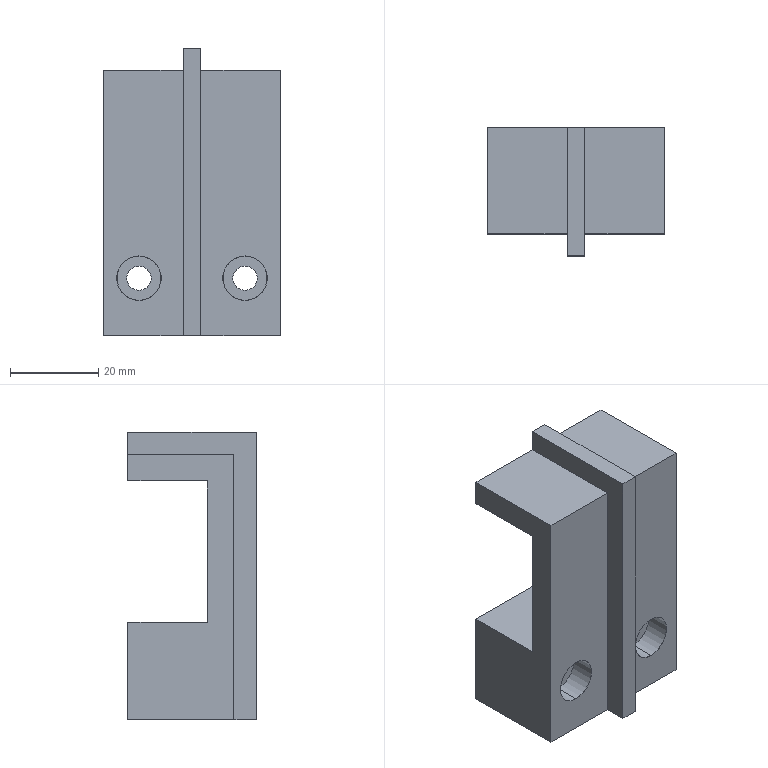Part | SolidWorks | features ICE 5, Extrusion 1, HoleWzd 1 | 1 solid | 30 faces | box 40 x 29 x 65 mm | volume 34575 mm3 | plane 18 | cylinder 8 | cone 4 | commonest cylinder face diameters 5.5 x4 10 x4
STEP:
#1=CARTESIAN_POINT('',(12.,0.025,-12.));
#2=VERTEX_POINT('',#1);
#3=CARTESIAN_POINT('',(12.,0.025,-22.));
#4=VERTEX_POINT('',#3);
#5=CARTESIAN_POINT('',(12.,0.025,-17.));
#6=DIRECTION('',(0.,-1.,0.));
#7=DIRECTION('',(0.,0.,-1.));
#8=AXIS2_PLACEMENT_3D('',#5,#6,#7);
#9=CIRCLE('',#8,5.);
#10=EDGE_CURVE('',#2,#4,#9,.T.);
#11=ORIENTED_EDGE('',*,*,#10,.F.);
#12=CARTESIAN_POINT('',(12.,0.,-11.975));
#13=VERTEX_POINT('',#12);
#14=CARTESIAN_POINT('',(12.,0.,-11.975));
#15=DIRECTION('',(0.,-0.7071,0.7071));
#16=VECTOR('',#15,1000.);
#17=LINE('',#14,#16);
#18=EDGE_CURVE('',#2,#13,#17,.T.);
#19=ORIENTED_EDGE('',*,*,#18,.T.);
#20=CARTESIAN_POINT('',(12.,0.,-22.025));
#21=VERTEX_POINT('',#20);
#22=CARTESIAN_POINT('',(12.,0.,-17.));
#23=DIRECTION('',(0.,-1.,0.));
#24=DIRECTION('',(0.,0.,-1.));
#25=AXIS2_PLACEMENT_3D('',#22,#23,#24);
#26=CIRCLE('',#25,5.025);
#27=EDGE_CURVE('',#13,#21,#26,.T.);
#28=ORIENTED_EDGE('',*,*,#27,.T.);
#29=CARTESIAN_POINT('',(12.,0.,-22.025));
#30=DIRECTION('',(0.,-0.7071,-0.7071));
#31=VECTOR('',#30,1000.);
#32=LINE('',#29,#31);
#33=EDGE_CURVE('',#4,#21,#32,.T.);
#34=ORIENTED_EDGE('',*,*,#33,.F.);
#35=EDGE_LOOP('',(#11,#19,#28,#34));
#36=FACE_OUTER_BOUND('',#35,.T.);
#37=CARTESIAN_POINT('',(12.,0.,-17.));
#38=DIRECTION('',(0.,-1.,0.));
#39=DIRECTION('',(0.,0.,-1.));
#40=AXIS2_PLACEMENT_3D('',#37,#38,#39);
#41=CONICAL_SURFACE('',#40,5.025,0.7854);
#42=ADVANCED_FACE('',(#36),#41,.F.);
#43=CARTESIAN_POINT('',(12.,5.7,-12.));
#44=VERTEX_POINT('',#43);
#45=CARTESIAN_POINT('',(12.,5.7,-22.));
#46=VERTEX_POINT('',#45);
#47=CARTESIAN_POINT('',(12.,5.7,-17.));
#48=DIRECTION('',(0.,-1.,0.));
#49=DIRECTION('',(0.,0.,-1.));
#50=AXIS2_PLACEMENT_3D('',#47,#48,#49);
#51=CIRCLE('',#50,5.);
#52=EDGE_CURVE('',#44,#46,#51,.T.);
#53=ORIENTED_EDGE('',*,*,#52,.F.);
#54=CARTESIAN_POINT('',(12.,0.,-12.));
#55=DIRECTION('',(0.,-1.,0.));
#56=VECTOR('',#55,1000.);
#57=LINE('',#54,#56);
#58=EDGE_CURVE('',#44,#2,#57,.T.);
#59=ORIENTED_EDGE('',*,*,#58,.T.);
#60=ORIENTED_EDGE('',*,*,#10,.T.);
#61=CARTESIAN_POINT('',(12.,0.,-22.));
#62=DIRECTION('',(0.,-1.,0.));
#63=VECTOR('',#62,1000.);
#64=LINE('',#61,#63);
#65=EDGE_CURVE('',#46,#4,#64,.T.);
#66=ORIENTED_EDGE('',*,*,#65,.F.);
#67=EDGE_LOOP('',(#53,#59,#60,#66));
#68=FACE_OUTER_BOUND('',#67,.T.);
#69=CARTESIAN_POINT('',(12.,0.,-17.));
#70=DIRECTION('',(0.,-1.,0.));
#71=DIRECTION('',(0.,0.,-1.));
#72=AXIS2_PLACEMENT_3D('',#69,#70,#71);
#73=CYLINDRICAL_SURFACE('',#72,5.);
#74=ADVANCED_FACE('',(#68),#73,.F.);
#75=CARTESIAN_POINT('',(12.,24.,-14.25));
#76=VERTEX_POINT('',#75);
#77=CARTESIAN_POINT('',(12.,24.,-19.75));
#78=VERTEX_POINT('',#77);
#79=CARTESIAN_POINT('',(12.,24.,-17.));
#80=DIRECTION('',(0.,-1.,0.));
#81=DIRECTION('',(0.,0.,-1.));
#82=AXIS2_PLACEMENT_3D('',#79,#80,#81);
#83=CIRCLE('',#82,2.75);
#84=EDGE_CURVE('',#76,#78,#83,.T.);
#85=ORIENTED_EDGE('',*,*,#84,.F.);
#86=CARTESIAN_POINT('',(12.,5.7,-14.25));
#87=VERTEX_POINT('',#86);
#88=CARTESIAN_POINT('',(12.,0.,-14.25));
#89=DIRECTION('',(0.,-1.,0.));
#90=VECTOR('',#89,1000.);
#91=LINE('',#88,#90);
#92=EDGE_CURVE('',#76,#87,#91,.T.);
#93=ORIENTED_EDGE('',*,*,#92,.T.);
#94=CARTESIAN_POINT('',(12.,5.7,-19.75));
#95=VERTEX_POINT('',#94);
#96=CARTESIAN_POINT('',(12.,5.7,-17.));
#97=DIRECTION('',(0.,-1.,0.));
#98=DIRECTION('',(0.,0.,-1.));
#99=AXIS2_PLACEMENT_3D('',#96,#97,#98);
#100=CIRCLE('',#99,2.75);
#101=EDGE_CURVE('',#87,#95,#100,.T.);
#102=ORIENTED_EDGE('',*,*,#101,.T.);
#103=CARTESIAN_POINT('',(12.,0.,-19.75));
#104=DIRECTION('',(0.,-1.,0.));
#105=VECTOR('',#104,1000.);
#106=LINE('',#103,#105);
#107=EDGE_CURVE('',#78,#95,#106,.T.);
#108=ORIENTED_EDGE('',*,*,#107,.F.);
#109=EDGE_LOOP('',(#85,#93,#102,#108));
#110=FACE_OUTER_BOUND('',#109,.T.);
#111=CARTESIAN_POINT('',(12.,0.,-17.));
#112=DIRECTION('',(0.,-1.,0.));
#113=DIRECTION('',(0.,0.,-1.));
#114=AXIS2_PLACEMENT_3D('',#111,#112,#113);
#115=CYLINDRICAL_SURFACE('',#114,2.75);
#116=ADVANCED_FACE('',(#110),#115,.F.);
#117=CARTESIAN_POINT('',(-12.,0.025,-12.));
#118=VERTEX_POINT('',#117);
#119=CARTESIAN_POINT('',(-12.,0.025,-22.));
#120=VERTEX_POINT('',#119);
#121=CARTESIAN_POINT('',(-12.,0.025,-17.));
#122=DIRECTION('',(0.,-1.,0.));
#123=DIRECTION('',(0.,0.,-1.));
#124=AXIS2_PLACEMENT_3D('',#121,#122,#123);
#125=CIRCLE('',#124,5.);
#126=EDGE_CURVE('',#118,#120,#125,.T.);
#127=ORIENTED_EDGE('',*,*,#126,.F.);
#128=CARTESIAN_POINT('',(-12.,0.,-11.975));
#129=VERTEX_POINT('',#128);
#130=CARTESIAN_POINT('',(-12.,0.,-11.975));
#131=DIRECTION('',(0.,-0.7071,0.7071));
#132=VECTOR('',#131,1000.);
#133=LINE('',#130,#132);
#134=EDGE_CURVE('',#118,#129,#133,.T.);
#135=ORIENTED_EDGE('',*,*,#134,.T.);
#136=CARTESIAN_POINT('',(-12.,0.,-22.025));
#137=VERTEX_POINT('',#136);
#138=CARTESIAN_POINT('',(-12.,0.,-17.));
#139=DIRECTION('',(0.,-1.,0.));
#140=DIRECTION('',(0.,0.,-1.));
#141=AXIS2_PLACEMENT_3D('',#138,#139,#140);
#142=CIRCLE('',#141,5.025);
#143=EDGE_CURVE('',#129,#137,#142,.T.);
#144=ORIENTED_EDGE('',*,*,#143,.T.);
#145=CARTESIAN_POINT('',(-12.,0.,-22.025));
#146=DIRECTION('',(0.,-0.7071,-0.7071));
#147=VECTOR('',#146,1000.);
#148=LINE('',#145,#147);
#149=EDGE_CURVE('',#120,#137,#148,.T.);
#150=ORIENTED_EDGE('',*,*,#149,.F.);
#151=EDGE_LOOP('',(#127,#135,#144,#150));
#152=FACE_OUTER_BOUND('',#151,.T.);
#153=CARTESIAN_POINT('',(-12.,0.,-17.));
#154=DIRECTION('',(0.,-1.,0.));
#155=DIRECTION('',(0.,0.,-1.));
#156=AXIS2_PLACEMENT_3D('',#153,#154,#155);
#157=CONICAL_SURFACE('',#156,5.025,0.7854);
#158=ADVANCED_FACE('',(#152),#157,.F.);
#159=CARTESIAN_POINT('',(-12.,5.7,-12.));
#160=VERTEX_POINT('',#159);
#161=CARTESIAN_POINT('',(-12.,5.7,-22.));
#162=VERTEX_POINT('',#161);
#163=CARTESIAN_POINT('',(-12.,5.7,-17.));
#164=DIRECTION('',(0.,-1.,0.));
#165=DIRECTION('',(0.,0.,-1.));
#166=AXIS2_PLACEMENT_3D('',#163,#164,#165);
#167=CIRCLE('',#166,5.);
#168=EDGE_CURVE('',#160,#162,#167,.T.);
#169=ORIENTED_EDGE('',*,*,#168,.F.);
#170=CARTESIAN_POINT('',(-12.,0.,-12.));
#171=DIRECTION('',(0.,-1.,0.));
#172=VECTOR('',#171,1000.);
#173=LINE('',#170,#172);
#174=EDGE_CURVE('',#160,#118,#173,.T.);
#175=ORIENTED_EDGE('',*,*,#174,.T.);
#176=ORIENTED_EDGE('',*,*,#126,.T.);
#177=CARTESIAN_POINT('',(-12.,0.,-22.));
#178=DIRECTION('',(0.,-1.,0.));
#179=VECTOR('',#178,1000.);
#180=LINE('',#177,#179);
#181=EDGE_CURVE('',#162,#120,#180,.T.);
#182=ORIENTED_EDGE('',*,*,#181,.F.);
#183=EDGE_LOOP('',(#169,#175,#176,#182));
#184=FACE_OUTER_BOUND('',#183,.T.);
#185=CARTESIAN_POINT('',(-12.,0.,-17.));
#186=DIRECTION('',(0.,-1.,0.));
#187=DIRECTION('',(0.,0.,-1.));
#188=AXIS2_PLACEMENT_3D('',#185,#186,#187);
#189=CYLINDRICAL_SURFACE('',#188,5.);
#190=ADVANCED_FACE('',(#184),#189,.F.);
#191=CARTESIAN_POINT('',(-12.,24.,-14.25));
#192=VERTEX_POINT('',#191);
#193=CARTESIAN_POINT('',(-12.,24.,-19.75));
#194=VERTEX_POINT('',#193);
#195=CARTESIAN_POINT('',(-12.,24.,-17.));
#196=DIRECTION('',(0.,-1.,0.));
#197=DIRECTION('',(0.,0.,-1.));
#198=AXIS2_PLACEMENT_3D('',#195,#196,#197);
#199=CIRCLE('',#198,2.75);
#200=EDGE_CURVE('',#192,#194,#199,.T.);
#201=ORIENTED_EDGE('',*,*,#200,.F.);
#202=CARTESIAN_POINT('',(-12.,5.7,-14.25));
#203=VERTEX_POINT('',#202);
#204=CARTESIAN_POINT('',(-12.,0.,-14.25));
#205=DIRECTION('',(0.,-1.,0.));
#206=VECTOR('',#205,1000.);
#207=LINE('',#204,#206);
#208=EDGE_CURVE('',#192,#203,#207,.T.);
#209=ORIENTED_EDGE('',*,*,#208,.T.);
#210=CARTESIAN_POINT('',(-12.,5.7,-19.75));
#211=VERTEX_POINT('',#210);
#212=CARTESIAN_POINT('',(-12.,5.7,-17.));
#213=DIRECTION('',(0.,-1.,0.));
#214=DIRECTION('',(0.,0.,-1.));
#215=AXIS2_PLACEMENT_3D('',#212,#213,#214);
#216=CIRCLE('',#215,2.75);
#217=EDGE_CURVE('',#203,#211,#216,.T.);
#218=ORIENTED_EDGE('',*,*,#217,.T.);
#219=CARTESIAN_POINT('',(-12.,0.,-19.75));
#220=DIRECTION('',(0.,-1.,0.));
#221=VECTOR('',#220,1000.);
#222=LINE('',#219,#221);
#223=EDGE_CURVE('',#194,#211,#222,.T.);
#224=ORIENTED_EDGE('',*,*,#223,.F.);
#225=EDGE_LOOP('',(#201,#209,#218,#224));
#226=FACE_OUTER_BOUND('',#225,.T.);
#227=CARTESIAN_POINT('',(-12.,0.,-17.));
#228=DIRECTION('',(0.,-1.,0.));
#229=DIRECTION('',(0.,0.,-1.));
#230=AXIS2_PLACEMENT_3D('',#227,#228,#229);
#231=CYLINDRICAL_SURFACE('',#230,2.75);
#232=ADVANCED_FACE('',(#226),#231,.F.);
#233=CARTESIAN_POINT('',(-2.,24.,30.));
#234=VERTEX_POINT('',#233);
#235=CARTESIAN_POINT('',(-2.,0.,30.));
#236=VERTEX_POINT('',#235);
#237=CARTESIAN_POINT('',(-2.,-5.,30.));
#238=DIRECTION('',(0.,-1.,0.));
#239=VECTOR('',#238,1000.);
#240=LINE('',#237,#239);
#241=EDGE_CURVE('',#234,#236,#240,.T.);
#242=ORIENTED_EDGE('',*,*,#241,.F.);
#243=CARTESIAN_POINT('',(-20.,24.,30.));
#244=VERTEX_POINT('',#243);
#245=CARTESIAN_POINT('',(-20.,24.,30.));
#246=DIRECTION('',(-1.,0.,0.));
#247=VECTOR('',#246,1000.);
#248=LINE('',#245,#247);
#249=EDGE_CURVE('',#234,#244,#248,.T.);
#250=ORIENTED_EDGE('',*,*,#249,.T.);
#251=CARTESIAN_POINT('',(-20.,0.,30.));
#252=VERTEX_POINT('',#251);
#253=CARTESIAN_POINT('',(-20.,24.,30.));
#254=DIRECTION('',(0.,-1.,0.));
#255=VECTOR('',#254,1000.);
#256=LINE('',#253,#255);
#257=EDGE_CURVE('',#244,#252,#256,.T.);
#258=ORIENTED_EDGE('',*,*,#257,.T.);
#259=CARTESIAN_POINT('',(-20.,0.,30.));
#260=DIRECTION('',(1.,0.,0.));
#261=VECTOR('',#260,1000.);
#262=LINE('',#259,#261);
#263=EDGE_CURVE('',#252,#236,#262,.T.);
#264=ORIENTED_EDGE('',*,*,#263,.T.);
#265=EDGE_LOOP('',(#242,#250,#258,#264));
#266=FACE_OUTER_BOUND('',#265,.T.);
#267=CARTESIAN_POINT('',(-20.,24.,30.));
#268=DIRECTION('',(0.,0.,-1.));
#269=DIRECTION('',(-1.,0.,0.));
#270=AXIS2_PLACEMENT_3D('',#267,#268,#269);
#271=PLANE('',#270);
#272=ADVANCED_FACE('',(#266),#271,.F.);
#273=CARTESIAN_POINT('',(20.,24.,30.));
#274=VERTEX_POINT('',#273);
#275=CARTESIAN_POINT('',(2.,24.,30.));
#276=VERTEX_POINT('',#275);
#277=CARTESIAN_POINT('',(-20.,24.,30.));
#278=DIRECTION('',(-1.,0.,0.));
#279=VECTOR('',#278,1000.);
#280=LINE('',#277,#279);
#281=EDGE_CURVE('',#274,#276,#280,.T.);
#282=ORIENTED_EDGE('',*,*,#281,.T.);
#283=CARTESIAN_POINT('',(2.,0.,30.));
#284=VERTEX_POINT('',#283);
#285=CARTESIAN_POINT('',(2.,-5.,30.));
#286=DIRECTION('',(0.,1.,0.));
#287=VECTOR('',#286,1000.);
#288=LINE('',#285,#287);
#289=EDGE_CURVE('',#284,#276,#288,.T.);
#290=ORIENTED_EDGE('',*,*,#289,.F.);
#291=CARTESIAN_POINT('',(20.,0.,30.));
#292=VERTEX_POINT('',#291);
#293=CARTESIAN_POINT('',(-20.,0.,30.));
#294=DIRECTION('',(1.,0.,0.));
#295=VECTOR('',#294,1000.);
#296=LINE('',#293,#295);
#297=EDGE_CURVE('',#284,#292,#296,.T.);
#298=ORIENTED_EDGE('',*,*,#297,.T.);
#299=CARTESIAN_POINT('',(20.,24.,30.));
#300=DIRECTION('',(0.,-1.,0.));
#301=VECTOR('',#300,1000.);
#302=LINE('',#299,#301);
#303=EDGE_CURVE('',#274,#292,#302,.T.);
#304=ORIENTED_EDGE('',*,*,#303,.F.);
#305=EDGE_LOOP('',(#282,#290,#298,#304));
#306=FACE_OUTER_BOUND('',#305,.T.);
#307=CARTESIAN_POINT('',(-20.,24.,30.));
#308=DIRECTION('',(0.,0.,-1.));
#309=DIRECTION('',(-1.,0.,0.));
#310=AXIS2_PLACEMENT_3D('',#307,#308,#309);
#311=PLANE('',#310);
#312=ADVANCED_FACE('',(#306),#311,.F.);
#313=CARTESIAN_POINT('',(20.,6.,24.));
#314=VERTEX_POINT('',#313);
#315=CARTESIAN_POINT('',(-20.,6.,24.));
#316=VERTEX_POINT('',#315);
#317=CARTESIAN_POINT('',(-20.,6.,24.));
#318=DIRECTION('',(-1.,0.,0.));
#319=VECTOR('',#318,1000.);
#320=LINE('',#317,#319);
#321=EDGE_CURVE('',#314,#316,#320,.T.);
#322=ORIENTED_EDGE('',*,*,#321,.F.);
#323=CARTESIAN_POINT('',(20.,6.,-8.));
#324=VERTEX_POINT('',#323);
#325=CARTESIAN_POINT('',(20.,6.,30.));
#326=DIRECTION('',(0.,0.,1.));
#327=VECTOR('',#326,1000.);
#328=LINE('',#325,#327);
#329=EDGE_CURVE('',#324,#314,#328,.T.);
#330=ORIENTED_EDGE('',*,*,#329,.F.);
#331=CARTESIAN_POINT('',(-20.,6.,-8.));
#332=VERTEX_POINT('',#331);
#333=CARTESIAN_POINT('',(63.,6.,-8.));
#334=DIRECTION('',(-1.,0.,0.));
#335=VECTOR('',#334,1000.);
#336=LINE('',#333,#335);
#337=EDGE_CURVE('',#324,#332,#336,.T.);
#338=ORIENTED_EDGE('',*,*,#337,.T.);
#339=CARTESIAN_POINT('',(-20.,6.,30.));
#340=DIRECTION('',(0.,0.,1.));
#341=VECTOR('',#340,1000.);
#342=LINE('',#339,#341);
#343=EDGE_CURVE('',#332,#316,#342,.T.);
#344=ORIENTED_EDGE('',*,*,#343,.T.);
#345=EDGE_LOOP('',(#322,#330,#338,#344));
#346=FACE_OUTER_BOUND('',#345,.T.);
#347=CARTESIAN_POINT('',(63.,6.,30.));
#348=DIRECTION('',(0.,-1.,0.));
#349=DIRECTION('',(0.,0.,-1.));
#350=AXIS2_PLACEMENT_3D('',#347,#348,#349);
#351=PLANE('',#350);
#352=ADVANCED_FACE('',(#346),#351,.F.);
#353=CARTESIAN_POINT('',(12.,0.,-17.));
#354=DIRECTION('',(0.,-1.,0.));
#355=DIRECTION('',(0.,0.,-1.));
#356=AXIS2_PLACEMENT_3D('',#353,#354,#355);
#357=CIRCLE('',#356,5.025);
#358=EDGE_CURVE('',#21,#13,#357,.T.);
#359=ORIENTED_EDGE('',*,*,#358,.F.);
#360=ORIENTED_EDGE('',*,*,#27,.F.);
#361=EDGE_LOOP('',(#359,#360));
#362=FACE_BOUND('',#361,.T.);
#363=CARTESIAN_POINT('',(2.,0.,-30.));
#364=VERTEX_POINT('',#363);
#365=CARTESIAN_POINT('',(2.,0.,-30.));
#366=DIRECTION('',(0.,0.,1.));
#367=VECTOR('',#366,1000.);
#368=LINE('',#365,#367);
#369=EDGE_CURVE('',#364,#284,#368,.T.);
#370=ORIENTED_EDGE('',*,*,#369,.F.);
#371=CARTESIAN_POINT('',(20.,0.,-30.));
#372=VERTEX_POINT('',#371);
#373=CARTESIAN_POINT('',(-20.,0.,-30.));
#374=DIRECTION('',(-1.,0.,0.));
#375=VECTOR('',#374,1000.);
#376=LINE('',#373,#375);
#377=EDGE_CURVE('',#372,#364,#376,.T.);
#378=ORIENTED_EDGE('',*,*,#377,.F.);
#379=CARTESIAN_POINT('',(20.,0.,30.));
#380=DIRECTION('',(0.,0.,-1.));
#381=VECTOR('',#380,1000.);
#382=LINE('',#379,#381);
#383=EDGE_CURVE('',#292,#372,#382,.T.);
#384=ORIENTED_EDGE('',*,*,#383,.F.);
#385=ORIENTED_EDGE('',*,*,#297,.F.);
#386=EDGE_LOOP('',(#370,#378,#384,#385));
#387=FACE_OUTER_BOUND('',#386,.T.);
#388=CARTESIAN_POINT('',(0.,0.,0.));
#389=DIRECTION('',(0.,-1.,0.));
#390=DIRECTION('',(0.,0.,-1.));
#391=AXIS2_PLACEMENT_3D('',#388,#389,#390);
#392=PLANE('',#391);
#393=ADVANCED_FACE('',(#362,#387),#392,.T.);
#394=CARTESIAN_POINT('',(20.,24.,-8.));
#395=VERTEX_POINT('',#394);
#396=CARTESIAN_POINT('',(20.,24.,-8.));
#397=DIRECTION('',(0.,-1.,0.));
#398=VECTOR('',#397,1000.);
#399=LINE('',#396,#398);
#400=EDGE_CURVE('',#395,#324,#399,.T.);
#401=ORIENTED_EDGE('',*,*,#400,.T.);
#402=ORIENTED_EDGE('',*,*,#329,.T.);
#403=CARTESIAN_POINT('',(20.,24.,24.));
#404=VERTEX_POINT('',#403);
#405=CARTESIAN_POINT('',(20.,64.447,24.));
#406=DIRECTION('',(0.,-1.,0.));
#407=VECTOR('',#406,1000.);
#408=LINE('',#405,#407);
#409=EDGE_CURVE('',#404,#314,#408,.T.);
#410=ORIENTED_EDGE('',*,*,#409,.F.);
#411=CARTESIAN_POINT('',(20.,24.,30.));
#412=DIRECTION('',(0.,0.,1.));
#413=VECTOR('',#412,1000.);
#414=LINE('',#411,#413);
#415=EDGE_CURVE('',#404,#274,#414,.T.);
#416=ORIENTED_EDGE('',*,*,#415,.T.);
#417=ORIENTED_EDGE('',*,*,#303,.T.);
#418=ORIENTED_EDGE('',*,*,#383,.T.);
#419=CARTESIAN_POINT('',(20.,24.,-30.));
#420=VERTEX_POINT('',#419);
#421=CARTESIAN_POINT('',(20.,24.,-30.));
#422=DIRECTION('',(0.,-1.,0.));
#423=VECTOR('',#422,1000.);
#424=LINE('',#421,#423);
#425=EDGE_CURVE('',#420,#372,#424,.T.);
#426=ORIENTED_EDGE('',*,*,#425,.F.);
#427=CARTESIAN_POINT('',(20.,24.,30.));
#428=DIRECTION('',(0.,0.,-1.));
#429=VECTOR('',#428,1000.);
#430=LINE('',#427,#429);
#431=EDGE_CURVE('',#395,#420,#430,.T.);
#432=ORIENTED_EDGE('',*,*,#431,.F.);
#433=EDGE_LOOP('',(#401,#402,#410,#416,#417,#418,#426,#432));
#434=FACE_OUTER_BOUND('',#433,.T.);
#435=CARTESIAN_POINT('',(20.,24.,30.));
#436=DIRECTION('',(-1.,0.,0.));
#437=DIRECTION('',(0.,0.,1.));
#438=AXIS2_PLACEMENT_3D('',#435,#436,#437);
#439=PLANE('',#438);
#440=ADVANCED_FACE('',(#434),#439,.F.);
#441=ORIENTED_EDGE('',*,*,#377,.T.);
#442=CARTESIAN_POINT('',(2.,-5.,-30.));
#443=VERTEX_POINT('',#442);
#444=CARTESIAN_POINT('',(2.,-5.,-30.));
#445=DIRECTION('',(0.,1.,0.));
#446=VECTOR('',#445,1000.);
#447=LINE('',#444,#446);
#448=EDGE_CURVE('',#443,#364,#447,.T.);
#449=ORIENTED_EDGE('',*,*,#448,.F.);
#450=CARTESIAN_POINT('',(-2.,-5.,-30.));
#451=VERTEX_POINT('',#450);
#452=CARTESIAN_POINT('',(-2.,-5.,-30.));
#453=DIRECTION('',(1.,0.,0.));
#454=VECTOR('',#453,1000.);
#455=LINE('',#452,#454);
#456=EDGE_CURVE('',#451,#443,#455,.T.);
#457=ORIENTED_EDGE('',*,*,#456,.F.);
#458=CARTESIAN_POINT('',(-2.,0.,-30.));
#459=VERTEX_POINT('',#458);
#460=CARTESIAN_POINT('',(-2.,-5.,-30.));
#461=DIRECTION('',(0.,1.,0.));
#462=VECTOR('',#461,1000.);
#463=LINE('',#460,#462);
#464=EDGE_CURVE('',#451,#459,#463,.T.);
#465=ORIENTED_EDGE('',*,*,#464,.T.);
#466=CARTESIAN_POINT('',(-20.,0.,-30.));
#467=VERTEX_POINT('',#466);
#468=CARTESIAN_POINT('',(-20.,0.,-30.));
#469=DIRECTION('',(-1.,0.,0.));
#470=VECTOR('',#469,1000.);
#471=LINE('',#468,#470);
#472=EDGE_CURVE('',#459,#467,#471,.T.);
#473=ORIENTED_EDGE('',*,*,#472,.T.);
#474=CARTESIAN_POINT('',(-20.,24.,-30.));
#475=VERTEX_POINT('',#474);
#476=CARTESIAN_POINT('',(-20.,24.,-30.));
#477=DIRECTION('',(0.,-1.,0.));
#478=VECTOR('',#477,1000.);
#479=LINE('',#476,#478);
#480=EDGE_CURVE('',#475,#467,#479,.T.);
#481=ORIENTED_EDGE('',*,*,#480,.F.);
#482=CARTESIAN_POINT('',(-20.,24.,-30.));
#483=DIRECTION('',(-1.,0.,0.));
#484=VECTOR('',#483,1000.);
#485=LINE('',#482,#484);
#486=EDGE_CURVE('',#420,#475,#485,.T.);
#487=ORIENTED_EDGE('',*,*,#486,.F.);
#488=ORIENTED_EDGE('',*,*,#425,.T.);
#489=EDGE_LOOP('',(#441,#449,#457,#465,#473,#481,#487,#488));
#490=FACE_OUTER_BOUND('',#489,.T.);
#491=CARTESIAN_POINT('',(-20.,24.,-30.));
#492=DIRECTION('',(0.,0.,1.));
#493=DIRECTION('',(1.,0.,0.));
#494=AXIS2_PLACEMENT_3D('',#491,#492,#493);
#495=PLANE('',#494);
#496=ADVANCED_FACE('',(#490),#495,.F.);
#497=ORIENTED_EDGE('',*,*,#257,.F.);
#498=CARTESIAN_POINT('',(-20.,24.,24.));
#499=VERTEX_POINT('',#498);
#500=CARTESIAN_POINT('',(-20.,24.,30.));
#501=DIRECTION('',(0.,0.,-1.));
#502=VECTOR('',#501,1000.);
#503=LINE('',#500,#502);
#504=EDGE_CURVE('',#244,#499,#503,.T.);
#505=ORIENTED_EDGE('',*,*,#504,.T.);
#506=CARTESIAN_POINT('',(-20.,64.447,24.));
#507=DIRECTION('',(0.,-1.,0.));
#508=VECTOR('',#507,1000.);
#509=LINE('',#506,#508);
#510=EDGE_CURVE('',#499,#316,#509,.T.);
#511=ORIENTED_EDGE('',*,*,#510,.T.);
#512=ORIENTED_EDGE('',*,*,#343,.F.);
#513=CARTESIAN_POINT('',(-20.,24.,-8.));
#514=VERTEX_POINT('',#513);
#515=CARTESIAN_POINT('',(-20.,24.,-8.));
#516=DIRECTION('',(0.,-1.,0.));
#517=VECTOR('',#516,1000.);
#518=LINE('',#515,#517);
#519=EDGE_CURVE('',#514,#332,#518,.T.);
#520=ORIENTED_EDGE('',*,*,#519,.F.);
#521=CARTESIAN_POINT('',(-20.,24.,30.));
#522=DIRECTION('',(0.,0.,1.));
#523=VECTOR('',#522,1000.);
#524=LINE('',#521,#523);
#525=EDGE_CURVE('',#475,#514,#524,.T.);
#526=ORIENTED_EDGE('',*,*,#525,.F.);
#527=ORIENTED_EDGE('',*,*,#480,.T.);
#528=CARTESIAN_POINT('',(-20.,0.,30.));
#529=DIRECTION('',(0.,0.,1.));
#530=VECTOR('',#529,1000.);
#531=LINE('',#528,#530);
#532=EDGE_CURVE('',#467,#252,#531,.T.);
#533=ORIENTED_EDGE('',*,*,#532,.T.);
#534=EDGE_LOOP('',(#497,#505,#511,#512,#520,#526,#527,#533));
#535=FACE_OUTER_BOUND('',#534,.T.);
#536=CARTESIAN_POINT('',(-20.,24.,30.));
#537=DIRECTION('',(1.,0.,0.));
#538=DIRECTION('',(0.,0.,-1.));
#539=AXIS2_PLACEMENT_3D('',#536,#537,#538);
#540=PLANE('',#539);
#541=ADVANCED_FACE('',(#535),#540,.F.);
#542=CARTESIAN_POINT('',(12.,24.,-17.));
#543=DIRECTION('',(0.,-1.,0.));
#544=DIRECTION('',(0.,0.,-1.));
#545=AXIS2_PLACEMENT_3D('',#542,#543,#544);
#546=CIRCLE('',#545,2.75);
#547=EDGE_CURVE('',#78,#76,#546,.T.);
#548=ORIENTED_EDGE('',*,*,#547,.T.);
#549=ORIENTED_EDGE('',*,*,#84,.T.);
#550=EDGE_LOOP('',(#548,#549));
#551=FACE_BOUND('',#550,.T.);
#552=CARTESIAN_POINT('',(-12.,24.,-17.));
#553=DIRECTION('',(0.,-1.,0.));
#554=DIRECTION('',(0.,0.,-1.));
#555=AXIS2_PLACEMENT_3D('',#552,#553,#554);
#556=CIRCLE('',#555,2.75);
#557=EDGE_CURVE('',#194,#192,#556,.T.);
#558=ORIENTED_EDGE('',*,*,#557,.T.);
#559=ORIENTED_EDGE('',*,*,#200,.T.);
#560=EDGE_LOOP('',(#558,#559));
#561=FACE_BOUND('',#560,.T.);
#562=ORIENTED_EDGE('',*,*,#525,.T.);
#563=CARTESIAN_POINT('',(0.,24.,-8.));
#564=DIRECTION('',(1.,0.,0.));
#565=VECTOR('',#564,1000.);
#566=LINE('',#563,#565);
#567=EDGE_CURVE('',#514,#395,#566,.T.);
#568=ORIENTED_EDGE('',*,*,#567,.T.);
#569=ORIENTED_EDGE('',*,*,#431,.T.);
#570=ORIENTED_EDGE('',*,*,#486,.T.);
#571=EDGE_LOOP('',(#562,#568,#569,#570));
#572=FACE_OUTER_BOUND('',#571,.T.);
#573=CARTESIAN_POINT('',(0.,24.,0.));
#574=DIRECTION('',(0.,-1.,0.));
#575=DIRECTION('',(0.,0.,-1.));
#576=AXIS2_PLACEMENT_3D('',#573,#574,#575);
#577=PLANE('',#576);
#578=ADVANCED_FACE('',(#551,#561,#572),#577,.F.);
#579=CARTESIAN_POINT('',(-12.,0.,-17.));
#580=DIRECTION('',(0.,-1.,0.));
#581=DIRECTION('',(0.,0.,-1.));
#582=AXIS2_PLACEMENT_3D('',#579,#580,#581);
#583=CIRCLE('',#582,5.025);
#584=EDGE_CURVE('',#137,#129,#583,.T.);
#585=ORIENTED_EDGE('',*,*,#584,.F.);
#586=ORIENTED_EDGE('',*,*,#143,.F.);
#587=EDGE_LOOP('',(#585,#586));
#588=FACE_BOUND('',#587,.T.);
#589=CARTESIAN_POINT('',(-2.,0.,-30.));
#590=DIRECTION('',(0.,0.,-1.));
#591=VECTOR('',#590,1000.);
#592=LINE('',#589,#591);
#593=EDGE_CURVE('',#236,#459,#592,.T.);
#594=ORIENTED_EDGE('',*,*,#593,.F.);
#595=ORIENTED_EDGE('',*,*,#263,.F.);
#596=ORIENTED_EDGE('',*,*,#532,.F.);
#597=ORIENTED_EDGE('',*,*,#472,.F.);
#598=EDGE_LOOP('',(#594,#595,#596,#597));
#599=FACE_OUTER_BOUND('',#598,.T.);
#600=CARTESIAN_POINT('',(0.,0.,0.));
#601=DIRECTION('',(0.,-1.,0.));
#602=DIRECTION('',(0.,0.,-1.));
#603=AXIS2_PLACEMENT_3D('',#600,#601,#602);
#604=PLANE('',#603);
#605=ADVANCED_FACE('',(#588,#599),#604,.T.);
#606=ORIENTED_EDGE('',*,*,#567,.F.);
#607=ORIENTED_EDGE('',*,*,#519,.T.);
#608=ORIENTED_EDGE('',*,*,#337,.F.);
#609=ORIENTED_EDGE('',*,*,#400,.F.);
#610=EDGE_LOOP('',(#606,#607,#608,#609));
#611=FACE_OUTER_BOUND('',#610,.T.);
#612=CARTESIAN_POINT('',(63.,24.,-8.));
#613=DIRECTION('',(0.,0.,-1.));
#614=DIRECTION('',(0.,1.,0.));
#615=AXIS2_PLACEMENT_3D('',#612,#613,#614);
#616=PLANE('',#615);
#617=ADVANCED_FACE('',(#611),#616,.F.);
#618=ORIENTED_EDGE('',*,*,#369,.T.);
#619=ORIENTED_EDGE('',*,*,#289,.T.);
#620=CARTESIAN_POINT('',(2.,24.,35.));
#621=VERTEX_POINT('',#620);
#622=CARTESIAN_POINT('',(2.,24.,35.));
#623=DIRECTION('',(0.,0.,1.));
#624=VECTOR('',#623,1000.);
#625=LINE('',#622,#624);
#626=EDGE_CURVE('',#276,#621,#625,.T.);
#627=ORIENTED_EDGE('',*,*,#626,.T.);
#628=CARTESIAN_POINT('',(2.,-5.,35.));
#629=VERTEX_POINT('',#628);
#630=CARTESIAN_POINT('',(2.,-5.,35.));
#631=DIRECTION('',(0.,1.,0.));
#632=VECTOR('',#631,1000.);
#633=LINE('',#630,#632);
#634=EDGE_CURVE('',#629,#621,#633,.T.);
#635=ORIENTED_EDGE('',*,*,#634,.F.);
#636=CARTESIAN_POINT('',(2.,-5.,-30.));
#637=DIRECTION('',(0.,0.,1.));
#638=VECTOR('',#637,1000.);
#639=LINE('',#636,#638);
#640=EDGE_CURVE('',#443,#629,#639,.T.);
#641=ORIENTED_EDGE('',*,*,#640,.F.);
#642=ORIENTED_EDGE('',*,*,#448,.T.);
#643=EDGE_LOOP('',(#618,#619,#627,#635,#641,#642));
#644=FACE_OUTER_BOUND('',#643,.T.);
#645=CARTESIAN_POINT('',(2.,-5.,-30.));
#646=DIRECTION('',(-1.,0.,0.));
#647=DIRECTION('',(0.,0.,1.));
#648=AXIS2_PLACEMENT_3D('',#645,#646,#647);
#649=PLANE('',#648);
#650=ADVANCED_FACE('',(#644),#649,.F.);
#651=ORIENTED_EDGE('',*,*,#593,.T.);
#652=ORIENTED_EDGE('',*,*,#464,.F.);
#653=CARTESIAN_POINT('',(-2.,-5.,35.));
#654=VERTEX_POINT('',#653);
#655=CARTESIAN_POINT('',(-2.,-5.,-30.));
#656=DIRECTION('',(0.,0.,-1.));
#657=VECTOR('',#656,1000.);
#658=LINE('',#655,#657);
#659=EDGE_CURVE('',#654,#451,#658,.T.);
#660=ORIENTED_EDGE('',*,*,#659,.F.);
#661=CARTESIAN_POINT('',(-2.,24.,35.));
#662=VERTEX_POINT('',#661);
#663=CARTESIAN_POINT('',(-2.,-5.,35.));
#664=DIRECTION('',(0.,-1.,0.));
#665=VECTOR('',#664,1000.);
#666=LINE('',#663,#665);
#667=EDGE_CURVE('',#662,#654,#666,.T.);
#668=ORIENTED_EDGE('',*,*,#667,.F.);
#669=CARTESIAN_POINT('',(-2.,24.,30.));
#670=DIRECTION('',(0.,0.,-1.));
#671=VECTOR('',#670,1000.);
#672=LINE('',#669,#671);
#673=EDGE_CURVE('',#662,#234,#672,.T.);
#674=ORIENTED_EDGE('',*,*,#673,.T.);
#675=ORIENTED_EDGE('',*,*,#241,.T.);
#676=EDGE_LOOP('',(#651,#652,#660,#668,#674,#675));
#677=FACE_OUTER_BOUND('',#676,.T.);
#678=CARTESIAN_POINT('',(-2.,-5.,-30.));
#679=DIRECTION('',(1.,0.,0.));
#680=DIRECTION('',(0.,0.,-1.));
#681=AXIS2_PLACEMENT_3D('',#678,#679,#680);
#682=PLANE('',#681);
#683=ADVANCED_FACE('',(#677),#682,.F.);
#684=ORIENTED_EDGE('',*,*,#640,.T.);
#685=CARTESIAN_POINT('',(-2.,-5.,35.));
#686=DIRECTION('',(1.,0.,0.));
#687=VECTOR('',#686,1000.);
#688=LINE('',#685,#687);
#689=EDGE_CURVE('',#654,#629,#688,.T.);
#690=ORIENTED_EDGE('',*,*,#689,.F.);
#691=ORIENTED_EDGE('',*,*,#659,.T.);
#692=ORIENTED_EDGE('',*,*,#456,.T.);
#693=EDGE_LOOP('',(#684,#690,#691,#692));
#694=FACE_OUTER_BOUND('',#693,.T.);
#695=CARTESIAN_POINT('',(0.,-5.,0.));
#696=DIRECTION('',(0.,1.,0.));
#697=DIRECTION('',(0.,0.,1.));
#698=AXIS2_PLACEMENT_3D('',#695,#696,#697);
#699=PLANE('',#698);
#700=ADVANCED_FACE('',(#694),#699,.F.);
#701=ORIENTED_EDGE('',*,*,#667,.T.);
#702=ORIENTED_EDGE('',*,*,#689,.T.);
#703=ORIENTED_EDGE('',*,*,#634,.T.);
#704=CARTESIAN_POINT('',(-2.,24.,35.));
#705=DIRECTION('',(-1.,0.,0.));
#706=VECTOR('',#705,1000.);
#707=LINE('',#704,#706);
#708=EDGE_CURVE('',#621,#662,#707,.T.);
#709=ORIENTED_EDGE('',*,*,#708,.T.);
#710=EDGE_LOOP('',(#701,#702,#703,#709));
#711=FACE_OUTER_BOUND('',#710,.T.);
#712=CARTESIAN_POINT('',(0.,0.,35.));
#713=DIRECTION('',(0.,0.,-1.));
#714=DIRECTION('',(-1.,0.,0.));
#715=AXIS2_PLACEMENT_3D('',#712,#713,#714);
#716=PLANE('',#715);
#717=ADVANCED_FACE('',(#711),#716,.F.);
#718=ORIENTED_EDGE('',*,*,#510,.F.);
#719=CARTESIAN_POINT('',(-20.,24.,24.));
#720=DIRECTION('',(1.,0.,0.));
#721=VECTOR('',#720,1000.);
#722=LINE('',#719,#721);
#723=EDGE_CURVE('',#499,#404,#722,.T.);
#724=ORIENTED_EDGE('',*,*,#723,.T.);
#725=ORIENTED_EDGE('',*,*,#409,.T.);
#726=ORIENTED_EDGE('',*,*,#321,.T.);
#727=EDGE_LOOP('',(#718,#724,#725,#726));
#728=FACE_OUTER_BOUND('',#727,.T.);
#729=CARTESIAN_POINT('',(-20.,64.447,24.));
#730=DIRECTION('',(0.,0.,1.));
#731=DIRECTION('',(0.,-1.,0.));
#732=AXIS2_PLACEMENT_3D('',#729,#730,#731);
#733=PLANE('',#732);
#734=ADVANCED_FACE('',(#728),#733,.F.);
#735=ORIENTED_EDGE('',*,*,#281,.F.);
#736=ORIENTED_EDGE('',*,*,#415,.F.);
#737=ORIENTED_EDGE('',*,*,#723,.F.);
#738=ORIENTED_EDGE('',*,*,#504,.F.);
#739=ORIENTED_EDGE('',*,*,#249,.F.);
#740=ORIENTED_EDGE('',*,*,#673,.F.);
#741=ORIENTED_EDGE('',*,*,#708,.F.);
#742=ORIENTED_EDGE('',*,*,#626,.F.);
#743=EDGE_LOOP('',(#735,#736,#737,#738,#739,#740,#741,#742));
#744=FACE_OUTER_BOUND('',#743,.T.);
#745=CARTESIAN_POINT('',(0.,24.,0.));
#746=DIRECTION('',(0.,-1.,0.));
#747=DIRECTION('',(0.,0.,-1.));
#748=AXIS2_PLACEMENT_3D('',#745,#746,#747);
#749=PLANE('',#748);
#750=ADVANCED_FACE('',(#744),#749,.F.);
#751=ORIENTED_EDGE('',*,*,#208,.F.);
#752=ORIENTED_EDGE('',*,*,#557,.F.);
#753=ORIENTED_EDGE('',*,*,#223,.T.);
#754=CARTESIAN_POINT('',(-12.,5.7,-17.));
#755=DIRECTION('',(0.,-1.,0.));
#756=DIRECTION('',(0.,0.,-1.));
#757=AXIS2_PLACEMENT_3D('',#754,#755,#756);
#758=CIRCLE('',#757,2.75);
#759=EDGE_CURVE('',#211,#203,#758,.T.);
#760=ORIENTED_EDGE('',*,*,#759,.T.);
#761=EDGE_LOOP('',(#751,#752,#753,#760));
#762=FACE_OUTER_BOUND('',#761,.T.);
#763=CARTESIAN_POINT('',(-12.,0.,-17.));
#764=DIRECTION('',(0.,-1.,0.));
#765=DIRECTION('',(0.,0.,-1.));
#766=AXIS2_PLACEMENT_3D('',#763,#764,#765);
#767=CYLINDRICAL_SURFACE('',#766,2.75);
#768=ADVANCED_FACE('',(#762),#767,.F.);
#769=ORIENTED_EDGE('',*,*,#759,.F.);
#770=ORIENTED_EDGE('',*,*,#217,.F.);
#771=EDGE_LOOP('',(#769,#770));
#772=FACE_BOUND('',#771,.T.);
#773=CARTESIAN_POINT('',(-12.,5.7,-17.));
#774=DIRECTION('',(0.,-1.,0.));
#775=DIRECTION('',(0.,0.,-1.));
#776=AXIS2_PLACEMENT_3D('',#773,#774,#775);
#777=CIRCLE('',#776,5.);
#778=EDGE_CURVE('',#162,#160,#777,.T.);
#779=ORIENTED_EDGE('',*,*,#778,.T.);
#780=ORIENTED_EDGE('',*,*,#168,.T.);
#781=EDGE_LOOP('',(#779,#780));
#782=FACE_OUTER_BOUND('',#781,.T.);
#783=CARTESIAN_POINT('',(-7.,5.7,-17.));
#784=DIRECTION('',(0.,1.,0.));
#785=DIRECTION('',(0.,0.,1.));
#786=AXIS2_PLACEMENT_3D('',#783,#784,#785);
#787=PLANE('',#786);
#788=ADVANCED_FACE('',(#772,#782),#787,.F.);
#789=ORIENTED_EDGE('',*,*,#174,.F.);
#790=ORIENTED_EDGE('',*,*,#778,.F.);
#791=ORIENTED_EDGE('',*,*,#181,.T.);
#792=CARTESIAN_POINT('',(-12.,0.025,-17.));
#793=DIRECTION('',(0.,-1.,0.));
#794=DIRECTION('',(0.,0.,-1.));
#795=AXIS2_PLACEMENT_3D('',#792,#793,#794);
#796=CIRCLE('',#795,5.);
#797=EDGE_CURVE('',#120,#118,#796,.T.);
#798=ORIENTED_EDGE('',*,*,#797,.T.);
#799=EDGE_LOOP('',(#789,#790,#791,#798));
#800=FACE_OUTER_BOUND('',#799,.T.);
#801=CARTESIAN_POINT('',(-12.,0.,-17.));
#802=DIRECTION('',(0.,-1.,0.));
#803=DIRECTION('',(0.,0.,-1.));
#804=AXIS2_PLACEMENT_3D('',#801,#802,#803);
#805=CYLINDRICAL_SURFACE('',#804,5.);
#806=ADVANCED_FACE('',(#800),#805,.F.);
#807=ORIENTED_EDGE('',*,*,#134,.F.);
#808=ORIENTED_EDGE('',*,*,#797,.F.);
#809=ORIENTED_EDGE('',*,*,#149,.T.);
#810=ORIENTED_EDGE('',*,*,#584,.T.);
#811=EDGE_LOOP('',(#807,#808,#809,#810));
#812=FACE_OUTER_BOUND('',#811,.T.);
#813=CARTESIAN_POINT('',(-12.,0.,-17.));
#814=DIRECTION('',(0.,-1.,0.));
#815=DIRECTION('',(0.,0.,-1.));
#816=AXIS2_PLACEMENT_3D('',#813,#814,#815);
#817=CONICAL_SURFACE('',#816,5.025,0.7854);
#818=ADVANCED_FACE('',(#812),#817,.F.);
#819=ORIENTED_EDGE('',*,*,#92,.F.);
#820=ORIENTED_EDGE('',*,*,#547,.F.);
#821=ORIENTED_EDGE('',*,*,#107,.T.);
#822=CARTESIAN_POINT('',(12.,5.7,-17.));
#823=DIRECTION('',(0.,-1.,0.));
#824=DIRECTION('',(0.,0.,-1.));
#825=AXIS2_PLACEMENT_3D('',#822,#823,#824);
#826=CIRCLE('',#825,2.75);
#827=EDGE_CURVE('',#95,#87,#826,.T.);
#828=ORIENTED_EDGE('',*,*,#827,.T.);
#829=EDGE_LOOP('',(#819,#820,#821,#828));
#830=FACE_OUTER_BOUND('',#829,.T.);
#831=CARTESIAN_POINT('',(12.,0.,-17.));
#832=DIRECTION('',(0.,-1.,0.));
#833=DIRECTION('',(0.,0.,-1.));
#834=AXIS2_PLACEMENT_3D('',#831,#832,#833);
#835=CYLINDRICAL_SURFACE('',#834,2.75);
#836=ADVANCED_FACE('',(#830),#835,.F.);
#837=ORIENTED_EDGE('',*,*,#827,.F.);
#838=ORIENTED_EDGE('',*,*,#101,.F.);
#839=EDGE_LOOP('',(#837,#838));
#840=FACE_BOUND('',#839,.T.);
#841=CARTESIAN_POINT('',(12.,5.7,-17.));
#842=DIRECTION('',(0.,-1.,0.));
#843=DIRECTION('',(0.,0.,-1.));
#844=AXIS2_PLACEMENT_3D('',#841,#842,#843);
#845=CIRCLE('',#844,5.);
#846=EDGE_CURVE('',#46,#44,#845,.T.);
#847=ORIENTED_EDGE('',*,*,#846,.T.);
#848=ORIENTED_EDGE('',*,*,#52,.T.);
#849=EDGE_LOOP('',(#847,#848));
#850=FACE_OUTER_BOUND('',#849,.T.);
#851=CARTESIAN_POINT('',(17.,5.7,-17.));
#852=DIRECTION('',(0.,1.,0.));
#853=DIRECTION('',(0.,0.,1.));
#854=AXIS2_PLACEMENT_3D('',#851,#852,#853);
#855=PLANE('',#854);
#856=ADVANCED_FACE('',(#840,#850),#855,.F.);
#857=ORIENTED_EDGE('',*,*,#58,.F.);
#858=ORIENTED_EDGE('',*,*,#846,.F.);
#859=ORIENTED_EDGE('',*,*,#65,.T.);
#860=CARTESIAN_POINT('',(12.,0.025,-17.));
#861=DIRECTION('',(0.,-1.,0.));
#862=DIRECTION('',(0.,0.,-1.));
#863=AXIS2_PLACEMENT_3D('',#860,#861,#862);
#864=CIRCLE('',#863,5.);
#865=EDGE_CURVE('',#4,#2,#864,.T.);
#866=ORIENTED_EDGE('',*,*,#865,.T.);
#867=EDGE_LOOP('',(#857,#858,#859,#866));
#868=FACE_OUTER_BOUND('',#867,.T.);
#869=CARTESIAN_POINT('',(12.,0.,-17.));
#870=DIRECTION('',(0.,-1.,0.));
#871=DIRECTION('',(0.,0.,-1.));
#872=AXIS2_PLACEMENT_3D('',#869,#870,#871);
#873=CYLINDRICAL_SURFACE('',#872,5.);
#874=ADVANCED_FACE('',(#868),#873,.F.);
#875=ORIENTED_EDGE('',*,*,#18,.F.);
#876=ORIENTED_EDGE('',*,*,#865,.F.);
#877=ORIENTED_EDGE('',*,*,#33,.T.);
#878=ORIENTED_EDGE('',*,*,#358,.T.);
#879=EDGE_LOOP('',(#875,#876,#877,#878));
#880=FACE_OUTER_BOUND('',#879,.T.);
#881=CARTESIAN_POINT('',(12.,0.,-17.));
#882=DIRECTION('',(0.,-1.,0.));
#883=DIRECTION('',(0.,0.,-1.));
#884=AXIS2_PLACEMENT_3D('',#881,#882,#883);
#885=CONICAL_SURFACE('',#884,5.025,0.7854);
#886=ADVANCED_FACE('',(#880),#885,.F.);
#887=CLOSED_SHELL('',(#42,#74,#116,#158,#190,#232,#272,#312,#352,#393,#440,#496,#541,#578,#605,#617,#650,#683,#700,#717,#734,#750,#768,#788,#806,#818,#836,#856,#874,#886));
#888=MANIFOLD_SOLID_BREP('',#887);
#889=CARTESIAN_POINT('',(0.,0.,0.));
#890=DIRECTION('',(0.,0.,1.));
#891=DIRECTION('',(1.,0.,0.));
#892=AXIS2_PLACEMENT_3D('',#889,#890,#891);
#893=(LENGTH_UNIT()NAMED_UNIT(*)SI_UNIT(.MILLI.,.METRE.));
#894=UNCERTAINTY_MEASURE_WITH_UNIT(LENGTH_MEASURE(0.00001),#893,'','');
#895=(NAMED_UNIT(*)PLANE_ANGLE_UNIT()SI_UNIT($,.RADIAN.));
#896=(NAMED_UNIT(*)SI_UNIT($,.STERADIAN.)SOLID_ANGLE_UNIT());
#897=(GEOMETRIC_REPRESENTATION_CONTEXT(3)GLOBAL_UNCERTAINTY_ASSIGNED_CONTEXT((#894))GLOBAL_UNIT_ASSIGNED_CONTEXT((#893,#895,#896))REPRESENTATION_CONTEXT('',''));
#898=ADVANCED_BREP_SHAPE_REPRESENTATION('',(#888,#892),#897);